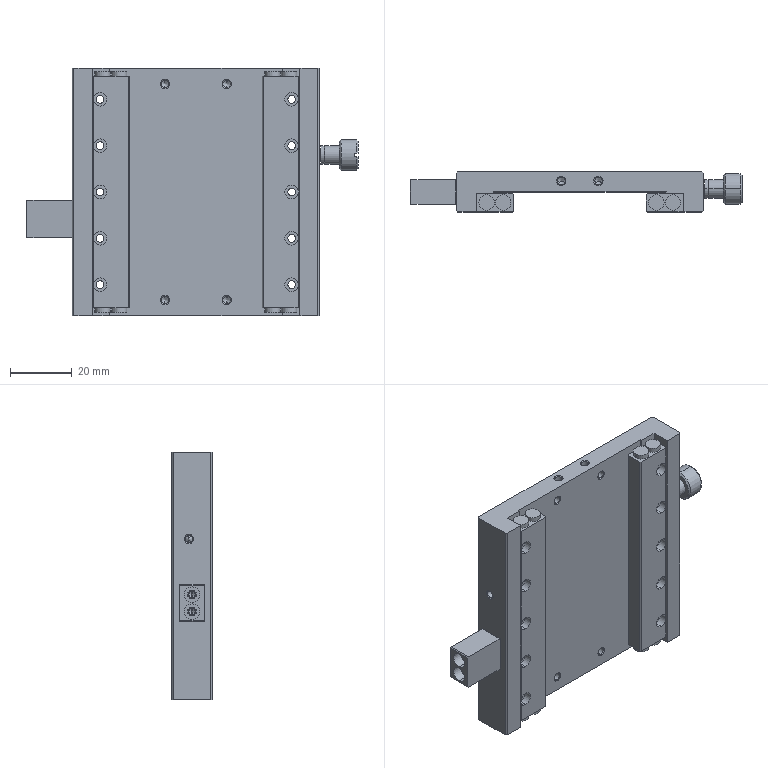Part | STEP file | E-EIC31-80-001 | 1 solid | 396 faces | box 107.5 x 13 x 80 mm | volume 58649 mm3 | cylinder 172 | cone 124 | plane 100 | commonest cylinder face diameters 2.459 x46 3.242 x26 6 x24 3.2 x20 4.4 x20 5 x20